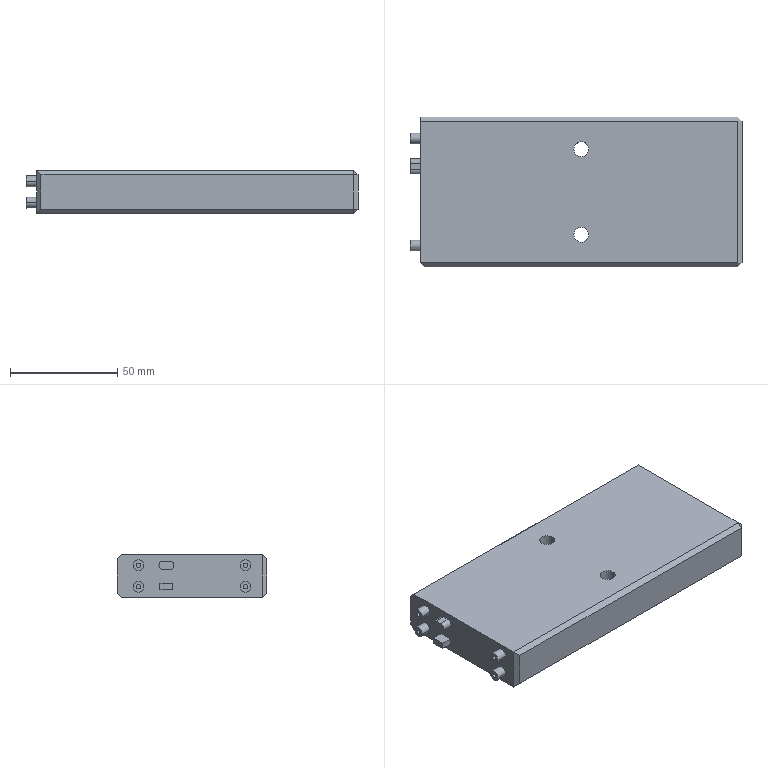Part | SolidWorks | features ICE 2, Chamfer 1, Extrusion 1 | 1 solid | 58 faces | box 155 x 70 x 20 mm | volume 207430 mm3 | plane 35 | cylinder 23 | commonest cylinder face diameters 2 x8 5 x8 7 x4 4 x3
STEP:
#1=CARTESIAN_POINT('',(-3.5,20.,-10.));
#2=VERTEX_POINT('',#1);
#3=CARTESIAN_POINT('',(3.5,20.,-10.));
#4=VERTEX_POINT('',#3);
#5=CARTESIAN_POINT('',(0.,20.,-10.));
#6=DIRECTION('',(0.,0.,1.));
#7=DIRECTION('',(1.,0.,0.));
#8=AXIS2_PLACEMENT_3D('',#5,#6,#7);
#9=CIRCLE('',#8,3.5);
#10=EDGE_CURVE('',#2,#4,#9,.T.);
#11=ORIENTED_EDGE('',*,*,#10,.F.);
#12=CARTESIAN_POINT('',(-3.5,20.,10.));
#13=VERTEX_POINT('',#12);
#14=CARTESIAN_POINT('',(-3.5,20.,-10.));
#15=DIRECTION('',(0.,0.,1.));
#16=VECTOR('',#15,1000.);
#17=LINE('',#14,#16);
#18=EDGE_CURVE('',#2,#13,#17,.T.);
#19=ORIENTED_EDGE('',*,*,#18,.T.);
#20=CARTESIAN_POINT('',(3.5,20.,10.));
#21=VERTEX_POINT('',#20);
#22=CARTESIAN_POINT('',(0.,20.,10.));
#23=DIRECTION('',(0.,0.,1.));
#24=DIRECTION('',(1.,0.,0.));
#25=AXIS2_PLACEMENT_3D('',#22,#23,#24);
#26=CIRCLE('',#25,3.5);
#27=EDGE_CURVE('',#13,#21,#26,.T.);
#28=ORIENTED_EDGE('',*,*,#27,.T.);
#29=CARTESIAN_POINT('',(3.5,20.,-10.));
#30=DIRECTION('',(0.,0.,1.));
#31=VECTOR('',#30,1000.);
#32=LINE('',#29,#31);
#33=EDGE_CURVE('',#4,#21,#32,.T.);
#34=ORIENTED_EDGE('',*,*,#33,.F.);
#35=EDGE_LOOP('',(#11,#19,#28,#34));
#36=FACE_OUTER_BOUND('',#35,.T.);
#37=CARTESIAN_POINT('',(0.,20.,-10.));
#38=DIRECTION('',(0.,0.,1.));
#39=DIRECTION('',(1.,0.,0.));
#40=AXIS2_PLACEMENT_3D('',#37,#38,#39);
#41=CYLINDRICAL_SURFACE('',#40,3.5);
#42=ADVANCED_FACE('',(#36),#41,.F.);
#43=CARTESIAN_POINT('',(-3.5,-20.,-10.));
#44=VERTEX_POINT('',#43);
#45=CARTESIAN_POINT('',(3.5,-20.,-10.));
#46=VERTEX_POINT('',#45);
#47=CARTESIAN_POINT('',(0.,-20.,-10.));
#48=DIRECTION('',(0.,0.,1.));
#49=DIRECTION('',(1.,0.,0.));
#50=AXIS2_PLACEMENT_3D('',#47,#48,#49);
#51=CIRCLE('',#50,3.5);
#52=EDGE_CURVE('',#44,#46,#51,.T.);
#53=ORIENTED_EDGE('',*,*,#52,.F.);
#54=CARTESIAN_POINT('',(-3.5,-20.,10.));
#55=VERTEX_POINT('',#54);
#56=CARTESIAN_POINT('',(-3.5,-20.,-10.));
#57=DIRECTION('',(0.,0.,1.));
#58=VECTOR('',#57,1000.);
#59=LINE('',#56,#58);
#60=EDGE_CURVE('',#44,#55,#59,.T.);
#61=ORIENTED_EDGE('',*,*,#60,.T.);
#62=CARTESIAN_POINT('',(3.5,-20.,10.));
#63=VERTEX_POINT('',#62);
#64=CARTESIAN_POINT('',(0.,-20.,10.));
#65=DIRECTION('',(0.,0.,1.));
#66=DIRECTION('',(1.,0.,0.));
#67=AXIS2_PLACEMENT_3D('',#64,#65,#66);
#68=CIRCLE('',#67,3.5);
#69=EDGE_CURVE('',#55,#63,#68,.T.);
#70=ORIENTED_EDGE('',*,*,#69,.T.);
#71=CARTESIAN_POINT('',(3.5,-20.,-10.));
#72=DIRECTION('',(0.,0.,1.));
#73=VECTOR('',#72,1000.);
#74=LINE('',#71,#73);
#75=EDGE_CURVE('',#46,#63,#74,.T.);
#76=ORIENTED_EDGE('',*,*,#75,.F.);
#77=EDGE_LOOP('',(#53,#61,#70,#76));
#78=FACE_OUTER_BOUND('',#77,.T.);
#79=CARTESIAN_POINT('',(0.,-20.,-10.));
#80=DIRECTION('',(0.,0.,1.));
#81=DIRECTION('',(1.,0.,0.));
#82=AXIS2_PLACEMENT_3D('',#79,#80,#81);
#83=CYLINDRICAL_SURFACE('',#82,3.5);
#84=ADVANCED_FACE('',(#78),#83,.F.);
#85=CARTESIAN_POINT('',(-80.,15.414,5.));
#86=VERTEX_POINT('',#85);
#87=CARTESIAN_POINT('',(-80.,13.414,3.));
#88=VERTEX_POINT('',#87);
#89=CARTESIAN_POINT('',(-80.,13.414,5.));
#90=DIRECTION('',(-1.,0.,0.));
#91=DIRECTION('',(0.,-1.,0.));
#92=AXIS2_PLACEMENT_3D('',#89,#90,#91);
#93=CIRCLE('',#92,2.);
#94=EDGE_CURVE('',#86,#88,#93,.T.);
#95=ORIENTED_EDGE('',*,*,#94,.F.);
#96=CARTESIAN_POINT('',(-75.,15.414,5.));
#97=VERTEX_POINT('',#96);
#98=CARTESIAN_POINT('',(-80.,15.414,5.));
#99=DIRECTION('',(1.,0.,0.));
#100=VECTOR('',#99,1000.);
#101=LINE('',#98,#100);
#102=EDGE_CURVE('',#86,#97,#101,.T.);
#103=ORIENTED_EDGE('',*,*,#102,.T.);
#104=CARTESIAN_POINT('',(-75.,13.414,3.));
#105=VERTEX_POINT('',#104);
#106=CARTESIAN_POINT('',(-75.,13.414,5.));
#107=DIRECTION('',(-1.,0.,0.));
#108=DIRECTION('',(0.,-1.,0.));
#109=AXIS2_PLACEMENT_3D('',#106,#107,#108);
#110=CIRCLE('',#109,2.);
#111=EDGE_CURVE('',#97,#105,#110,.T.);
#112=ORIENTED_EDGE('',*,*,#111,.T.);
#113=CARTESIAN_POINT('',(-80.,13.414,3.));
#114=DIRECTION('',(1.,0.,0.));
#115=VECTOR('',#114,1000.);
#116=LINE('',#113,#115);
#117=EDGE_CURVE('',#88,#105,#116,.T.);
#118=ORIENTED_EDGE('',*,*,#117,.F.);
#119=EDGE_LOOP('',(#95,#103,#112,#118));
#120=FACE_OUTER_BOUND('',#119,.T.);
#121=CARTESIAN_POINT('',(-80.,13.414,5.));
#122=DIRECTION('',(1.,0.,0.));
#123=DIRECTION('',(0.,1.,0.));
#124=AXIS2_PLACEMENT_3D('',#121,#122,#123);
#125=CYLINDRICAL_SURFACE('',#124,2.);
#126=ADVANCED_FACE('',(#120),#125,.T.);
#127=CARTESIAN_POINT('',(-80.,26.,-5.));
#128=VERTEX_POINT('',#127);
#129=CARTESIAN_POINT('',(-80.,24.,-5.));
#130=VERTEX_POINT('',#129);
#131=CARTESIAN_POINT('',(-80.,25.,-5.));
#132=DIRECTION('',(-1.,0.,0.));
#133=DIRECTION('',(0.,1.,0.));
#134=AXIS2_PLACEMENT_3D('',#131,#132,#133);
#135=CIRCLE('',#134,1.);
#136=EDGE_CURVE('',#128,#130,#135,.T.);
#137=ORIENTED_EDGE('',*,*,#136,.T.);
#138=CARTESIAN_POINT('',(-75.,24.,-5.));
#139=VERTEX_POINT('',#138);
#140=CARTESIAN_POINT('',(-80.,24.,-5.));
#141=DIRECTION('',(1.,0.,0.));
#142=VECTOR('',#141,1000.);
#143=LINE('',#140,#142);
#144=EDGE_CURVE('',#130,#139,#143,.T.);
#145=ORIENTED_EDGE('',*,*,#144,.T.);
#146=CARTESIAN_POINT('',(-75.,26.,-5.));
#147=VERTEX_POINT('',#146);
#148=CARTESIAN_POINT('',(-75.,25.,-5.));
#149=DIRECTION('',(-1.,0.,0.));
#150=DIRECTION('',(0.,1.,0.));
#151=AXIS2_PLACEMENT_3D('',#148,#149,#150);
#152=CIRCLE('',#151,1.);
#153=EDGE_CURVE('',#147,#139,#152,.T.);
#154=ORIENTED_EDGE('',*,*,#153,.F.);
#155=CARTESIAN_POINT('',(-80.,26.,-5.));
#156=DIRECTION('',(1.,0.,0.));
#157=VECTOR('',#156,1000.);
#158=LINE('',#155,#157);
#159=EDGE_CURVE('',#128,#147,#158,.T.);
#160=ORIENTED_EDGE('',*,*,#159,.F.);
#161=EDGE_LOOP('',(#137,#145,#154,#160));
#162=FACE_OUTER_BOUND('',#161,.T.);
#163=CARTESIAN_POINT('',(-80.,25.,-5.));
#164=DIRECTION('',(1.,0.,0.));
#165=DIRECTION('',(0.,1.,0.));
#166=AXIS2_PLACEMENT_3D('',#163,#164,#165);
#167=CYLINDRICAL_SURFACE('',#166,1.);
#168=ADVANCED_FACE('',(#162),#167,.F.);
#169=CARTESIAN_POINT('',(-80.,22.5,-5.));
#170=VERTEX_POINT('',#169);
#171=CARTESIAN_POINT('',(-80.,27.5,-5.));
#172=VERTEX_POINT('',#171);
#173=CARTESIAN_POINT('',(-80.,25.,-5.));
#174=DIRECTION('',(-1.,0.,0.));
#175=DIRECTION('',(0.,1.,0.));
#176=AXIS2_PLACEMENT_3D('',#173,#174,#175);
#177=CIRCLE('',#176,2.5);
#178=EDGE_CURVE('',#170,#172,#177,.T.);
#179=ORIENTED_EDGE('',*,*,#178,.F.);
#180=CARTESIAN_POINT('',(-75.,22.5,-5.));
#181=VERTEX_POINT('',#180);
#182=CARTESIAN_POINT('',(-80.,22.5,-5.));
#183=DIRECTION('',(1.,0.,0.));
#184=VECTOR('',#183,1000.);
#185=LINE('',#182,#184);
#186=EDGE_CURVE('',#170,#181,#185,.T.);
#187=ORIENTED_EDGE('',*,*,#186,.T.);
#188=CARTESIAN_POINT('',(-75.,27.5,-5.));
#189=VERTEX_POINT('',#188);
#190=CARTESIAN_POINT('',(-75.,25.,-5.));
#191=DIRECTION('',(-1.,0.,0.));
#192=DIRECTION('',(0.,1.,0.));
#193=AXIS2_PLACEMENT_3D('',#190,#191,#192);
#194=CIRCLE('',#193,2.5);
#195=EDGE_CURVE('',#181,#189,#194,.T.);
#196=ORIENTED_EDGE('',*,*,#195,.T.);
#197=CARTESIAN_POINT('',(-80.,27.5,-5.));
#198=DIRECTION('',(1.,0.,0.));
#199=VECTOR('',#198,1000.);
#200=LINE('',#197,#199);
#201=EDGE_CURVE('',#172,#189,#200,.T.);
#202=ORIENTED_EDGE('',*,*,#201,.F.);
#203=EDGE_LOOP('',(#179,#187,#196,#202));
#204=FACE_OUTER_BOUND('',#203,.T.);
#205=CARTESIAN_POINT('',(-80.,25.,-5.));
#206=DIRECTION('',(1.,0.,0.));
#207=DIRECTION('',(0.,1.,0.));
#208=AXIS2_PLACEMENT_3D('',#205,#206,#207);
#209=CYLINDRICAL_SURFACE('',#208,2.5);
#210=ADVANCED_FACE('',(#204),#209,.T.);
#211=CARTESIAN_POINT('',(-80.,26.,5.));
#212=VERTEX_POINT('',#211);
#213=CARTESIAN_POINT('',(-80.,24.,5.));
#214=VERTEX_POINT('',#213);
#215=CARTESIAN_POINT('',(-80.,25.,5.));
#216=DIRECTION('',(-1.,0.,0.));
#217=DIRECTION('',(0.,1.,0.));
#218=AXIS2_PLACEMENT_3D('',#215,#216,#217);
#219=CIRCLE('',#218,1.);
#220=EDGE_CURVE('',#212,#214,#219,.T.);
#221=ORIENTED_EDGE('',*,*,#220,.T.);
#222=CARTESIAN_POINT('',(-75.,24.,5.));
#223=VERTEX_POINT('',#222);
#224=CARTESIAN_POINT('',(-80.,24.,5.));
#225=DIRECTION('',(1.,0.,0.));
#226=VECTOR('',#225,1000.);
#227=LINE('',#224,#226);
#228=EDGE_CURVE('',#214,#223,#227,.T.);
#229=ORIENTED_EDGE('',*,*,#228,.T.);
#230=CARTESIAN_POINT('',(-75.,26.,5.));
#231=VERTEX_POINT('',#230);
#232=CARTESIAN_POINT('',(-75.,25.,5.));
#233=DIRECTION('',(-1.,0.,0.));
#234=DIRECTION('',(0.,1.,0.));
#235=AXIS2_PLACEMENT_3D('',#232,#233,#234);
#236=CIRCLE('',#235,1.);
#237=EDGE_CURVE('',#231,#223,#236,.T.);
#238=ORIENTED_EDGE('',*,*,#237,.F.);
#239=CARTESIAN_POINT('',(-80.,26.,5.));
#240=DIRECTION('',(1.,0.,0.));
#241=VECTOR('',#240,1000.);
#242=LINE('',#239,#241);
#243=EDGE_CURVE('',#212,#231,#242,.T.);
#244=ORIENTED_EDGE('',*,*,#243,.F.);
#245=EDGE_LOOP('',(#221,#229,#238,#244));
#246=FACE_OUTER_BOUND('',#245,.T.);
#247=CARTESIAN_POINT('',(-80.,25.,5.));
#248=DIRECTION('',(1.,0.,0.));
#249=DIRECTION('',(0.,1.,0.));
#250=AXIS2_PLACEMENT_3D('',#247,#248,#249);
#251=CYLINDRICAL_SURFACE('',#250,1.);
#252=ADVANCED_FACE('',(#246),#251,.F.);
#253=CARTESIAN_POINT('',(-80.,22.5,5.));
#254=VERTEX_POINT('',#253);
#255=CARTESIAN_POINT('',(-80.,27.5,5.));
#256=VERTEX_POINT('',#255);
#257=CARTESIAN_POINT('',(-80.,25.,5.));
#258=DIRECTION('',(-1.,0.,0.));
#259=DIRECTION('',(0.,1.,0.));
#260=AXIS2_PLACEMENT_3D('',#257,#258,#259);
#261=CIRCLE('',#260,2.5);
#262=EDGE_CURVE('',#254,#256,#261,.T.);
#263=ORIENTED_EDGE('',*,*,#262,.F.);
#264=CARTESIAN_POINT('',(-75.,22.5,5.));
#265=VERTEX_POINT('',#264);
#266=CARTESIAN_POINT('',(-80.,22.5,5.));
#267=DIRECTION('',(1.,0.,0.));
#268=VECTOR('',#267,1000.);
#269=LINE('',#266,#268);
#270=EDGE_CURVE('',#254,#265,#269,.T.);
#271=ORIENTED_EDGE('',*,*,#270,.T.);
#272=CARTESIAN_POINT('',(-75.,27.5,5.));
#273=VERTEX_POINT('',#272);
#274=CARTESIAN_POINT('',(-75.,25.,5.));
#275=DIRECTION('',(-1.,0.,0.));
#276=DIRECTION('',(0.,1.,0.));
#277=AXIS2_PLACEMENT_3D('',#274,#275,#276);
#278=CIRCLE('',#277,2.5);
#279=EDGE_CURVE('',#265,#273,#278,.T.);
#280=ORIENTED_EDGE('',*,*,#279,.T.);
#281=CARTESIAN_POINT('',(-80.,27.5,5.));
#282=DIRECTION('',(1.,0.,0.));
#283=VECTOR('',#282,1000.);
#284=LINE('',#281,#283);
#285=EDGE_CURVE('',#256,#273,#284,.T.);
#286=ORIENTED_EDGE('',*,*,#285,.F.);
#287=EDGE_LOOP('',(#263,#271,#280,#286));
#288=FACE_OUTER_BOUND('',#287,.T.);
#289=CARTESIAN_POINT('',(-80.,25.,5.));
#290=DIRECTION('',(1.,0.,0.));
#291=DIRECTION('',(0.,1.,0.));
#292=AXIS2_PLACEMENT_3D('',#289,#290,#291);
#293=CYLINDRICAL_SURFACE('',#292,2.5);
#294=ADVANCED_FACE('',(#288),#293,.T.);
#295=CARTESIAN_POINT('',(-80.,-24.,5.));
#296=VERTEX_POINT('',#295);
#297=CARTESIAN_POINT('',(-80.,-26.,5.));
#298=VERTEX_POINT('',#297);
#299=CARTESIAN_POINT('',(-80.,-25.,5.));
#300=DIRECTION('',(-1.,0.,0.));
#301=DIRECTION('',(0.,-1.,0.));
#302=AXIS2_PLACEMENT_3D('',#299,#300,#301);
#303=CIRCLE('',#302,1.);
#304=EDGE_CURVE('',#296,#298,#303,.T.);
#305=ORIENTED_EDGE('',*,*,#304,.T.);
#306=CARTESIAN_POINT('',(-75.,-26.,5.));
#307=VERTEX_POINT('',#306);
#308=CARTESIAN_POINT('',(-80.,-26.,5.));
#309=DIRECTION('',(1.,0.,0.));
#310=VECTOR('',#309,1000.);
#311=LINE('',#308,#310);
#312=EDGE_CURVE('',#298,#307,#311,.T.);
#313=ORIENTED_EDGE('',*,*,#312,.T.);
#314=CARTESIAN_POINT('',(-75.,-24.,5.));
#315=VERTEX_POINT('',#314);
#316=CARTESIAN_POINT('',(-75.,-25.,5.));
#317=DIRECTION('',(-1.,0.,0.));
#318=DIRECTION('',(0.,-1.,0.));
#319=AXIS2_PLACEMENT_3D('',#316,#317,#318);
#320=CIRCLE('',#319,1.);
#321=EDGE_CURVE('',#315,#307,#320,.T.);
#322=ORIENTED_EDGE('',*,*,#321,.F.);
#323=CARTESIAN_POINT('',(-80.,-24.,5.));
#324=DIRECTION('',(1.,0.,0.));
#325=VECTOR('',#324,1000.);
#326=LINE('',#323,#325);
#327=EDGE_CURVE('',#296,#315,#326,.T.);
#328=ORIENTED_EDGE('',*,*,#327,.F.);
#329=EDGE_LOOP('',(#305,#313,#322,#328));
#330=FACE_OUTER_BOUND('',#329,.T.);
#331=CARTESIAN_POINT('',(-80.,-25.,5.));
#332=DIRECTION('',(1.,0.,0.));
#333=DIRECTION('',(0.,1.,0.));
#334=AXIS2_PLACEMENT_3D('',#331,#332,#333);
#335=CYLINDRICAL_SURFACE('',#334,1.);
#336=ADVANCED_FACE('',(#330),#335,.F.);
#337=CARTESIAN_POINT('',(-80.,-27.5,5.));
#338=VERTEX_POINT('',#337);
#339=CARTESIAN_POINT('',(-80.,-22.5,5.));
#340=VERTEX_POINT('',#339);
#341=CARTESIAN_POINT('',(-80.,-25.,5.));
#342=DIRECTION('',(-1.,0.,0.));
#343=DIRECTION('',(0.,-1.,0.));
#344=AXIS2_PLACEMENT_3D('',#341,#342,#343);
#345=CIRCLE('',#344,2.5);
#346=EDGE_CURVE('',#338,#340,#345,.T.);
#347=ORIENTED_EDGE('',*,*,#346,.F.);
#348=CARTESIAN_POINT('',(-75.,-27.5,5.));
#349=VERTEX_POINT('',#348);
#350=CARTESIAN_POINT('',(-80.,-27.5,5.));
#351=DIRECTION('',(1.,0.,0.));
#352=VECTOR('',#351,1000.);
#353=LINE('',#350,#352);
#354=EDGE_CURVE('',#338,#349,#353,.T.);
#355=ORIENTED_EDGE('',*,*,#354,.T.);
#356=CARTESIAN_POINT('',(-75.,-22.5,5.));
#357=VERTEX_POINT('',#356);
#358=CARTESIAN_POINT('',(-75.,-25.,5.));
#359=DIRECTION('',(-1.,0.,0.));
#360=DIRECTION('',(0.,1.,0.));
#361=AXIS2_PLACEMENT_3D('',#358,#359,#360);
#362=CIRCLE('',#361,2.5);
#363=EDGE_CURVE('',#349,#357,#362,.T.);
#364=ORIENTED_EDGE('',*,*,#363,.T.);
#365=CARTESIAN_POINT('',(-80.,-22.5,5.));
#366=DIRECTION('',(1.,0.,0.));
#367=VECTOR('',#366,1000.);
#368=LINE('',#365,#367);
#369=EDGE_CURVE('',#340,#357,#368,.T.);
#370=ORIENTED_EDGE('',*,*,#369,.F.);
#371=EDGE_LOOP('',(#347,#355,#364,#370));
#372=FACE_OUTER_BOUND('',#371,.T.);
#373=CARTESIAN_POINT('',(-80.,-25.,5.));
#374=DIRECTION('',(1.,0.,0.));
#375=DIRECTION('',(0.,1.,0.));
#376=AXIS2_PLACEMENT_3D('',#373,#374,#375);
#377=CYLINDRICAL_SURFACE('',#376,2.5);
#378=ADVANCED_FACE('',(#372),#377,.T.);
#379=CARTESIAN_POINT('',(-80.,-24.,-5.));
#380=VERTEX_POINT('',#379);
#381=CARTESIAN_POINT('',(-80.,-26.,-5.));
#382=VERTEX_POINT('',#381);
#383=CARTESIAN_POINT('',(-80.,-25.,-5.));
#384=DIRECTION('',(-1.,0.,0.));
#385=DIRECTION('',(0.,-1.,0.));
#386=AXIS2_PLACEMENT_3D('',#383,#384,#385);
#387=CIRCLE('',#386,1.);
#388=EDGE_CURVE('',#380,#382,#387,.T.);
#389=ORIENTED_EDGE('',*,*,#388,.T.);
#390=CARTESIAN_POINT('',(-75.,-26.,-5.));
#391=VERTEX_POINT('',#390);
#392=CARTESIAN_POINT('',(-80.,-26.,-5.));
#393=DIRECTION('',(1.,0.,0.));
#394=VECTOR('',#393,1000.);
#395=LINE('',#392,#394);
#396=EDGE_CURVE('',#382,#391,#395,.T.);
#397=ORIENTED_EDGE('',*,*,#396,.T.);
#398=CARTESIAN_POINT('',(-75.,-24.,-5.));
#399=VERTEX_POINT('',#398);
#400=CARTESIAN_POINT('',(-75.,-25.,-5.));
#401=DIRECTION('',(-1.,0.,0.));
#402=DIRECTION('',(0.,-1.,0.));
#403=AXIS2_PLACEMENT_3D('',#400,#401,#402);
#404=CIRCLE('',#403,1.);
#405=EDGE_CURVE('',#399,#391,#404,.T.);
#406=ORIENTED_EDGE('',*,*,#405,.F.);
#407=CARTESIAN_POINT('',(-80.,-24.,-5.));
#408=DIRECTION('',(1.,0.,0.));
#409=VECTOR('',#408,1000.);
#410=LINE('',#407,#409);
#411=EDGE_CURVE('',#380,#399,#410,.T.);
#412=ORIENTED_EDGE('',*,*,#411,.F.);
#413=EDGE_LOOP('',(#389,#397,#406,#412));
#414=FACE_OUTER_BOUND('',#413,.T.);
#415=CARTESIAN_POINT('',(-80.,-25.,-5.));
#416=DIRECTION('',(1.,0.,0.));
#417=DIRECTION('',(0.,1.,0.));
#418=AXIS2_PLACEMENT_3D('',#415,#416,#417);
#419=CYLINDRICAL_SURFACE('',#418,1.);
#420=ADVANCED_FACE('',(#414),#419,.F.);
#421=CARTESIAN_POINT('',(-80.,-27.5,-5.));
#422=VERTEX_POINT('',#421);
#423=CARTESIAN_POINT('',(-80.,-22.5,-5.));
#424=VERTEX_POINT('',#423);
#425=CARTESIAN_POINT('',(-80.,-25.,-5.));
#426=DIRECTION('',(-1.,0.,0.));
#427=DIRECTION('',(0.,-1.,0.));
#428=AXIS2_PLACEMENT_3D('',#425,#426,#427);
#429=CIRCLE('',#428,2.5);
#430=EDGE_CURVE('',#422,#424,#429,.T.);
#431=ORIENTED_EDGE('',*,*,#430,.F.);
#432=CARTESIAN_POINT('',(-75.,-27.5,-5.));
#433=VERTEX_POINT('',#432);
#434=CARTESIAN_POINT('',(-80.,-27.5,-5.));
#435=DIRECTION('',(1.,0.,0.));
#436=VECTOR('',#435,1000.);
#437=LINE('',#434,#436);
#438=EDGE_CURVE('',#422,#433,#437,.T.);
#439=ORIENTED_EDGE('',*,*,#438,.T.);
#440=CARTESIAN_POINT('',(-75.,-22.5,-5.));
#441=VERTEX_POINT('',#440);
#442=CARTESIAN_POINT('',(-75.,-25.,-5.));
#443=DIRECTION('',(-1.,0.,0.));
#444=DIRECTION('',(0.,1.,0.));
#445=AXIS2_PLACEMENT_3D('',#442,#443,#444);
#446=CIRCLE('',#445,2.5);
#447=EDGE_CURVE('',#433,#441,#446,.T.);
#448=ORIENTED_EDGE('',*,*,#447,.T.);
#449=CARTESIAN_POINT('',(-80.,-22.5,-5.));
#450=DIRECTION('',(1.,0.,0.));
#451=VECTOR('',#450,1000.);
#452=LINE('',#449,#451);
#453=EDGE_CURVE('',#424,#441,#452,.T.);
#454=ORIENTED_EDGE('',*,*,#453,.F.);
#455=EDGE_LOOP('',(#431,#439,#448,#454));
#456=FACE_OUTER_BOUND('',#455,.T.);
#457=CARTESIAN_POINT('',(-80.,-25.,-5.));
#458=DIRECTION('',(1.,0.,0.));
#459=DIRECTION('',(0.,1.,0.));
#460=AXIS2_PLACEMENT_3D('',#457,#458,#459);
#461=CYLINDRICAL_SURFACE('',#460,2.5);
#462=ADVANCED_FACE('',(#456),#461,.T.);
#463=CARTESIAN_POINT('',(-75.,13.414,7.));
#464=VERTEX_POINT('',#463);
#465=CARTESIAN_POINT('',(-75.,13.414,5.));
#466=DIRECTION('',(-1.,0.,0.));
#467=DIRECTION('',(0.,-1.,0.));
#468=AXIS2_PLACEMENT_3D('',#465,#466,#467);
#469=CIRCLE('',#468,2.);
#470=EDGE_CURVE('',#464,#97,#469,.T.);
#471=ORIENTED_EDGE('',*,*,#470,.F.);
#472=CARTESIAN_POINT('',(-75.,10.414,7.));
#473=VERTEX_POINT('',#472);
#474=CARTESIAN_POINT('',(-75.,13.414,7.));
#475=DIRECTION('',(0.,1.,0.));
#476=VECTOR('',#475,1000.);
#477=LINE('',#474,#476);
#478=EDGE_CURVE('',#473,#464,#477,.T.);
#479=ORIENTED_EDGE('',*,*,#478,.F.);
#480=CARTESIAN_POINT('',(-75.,10.414,3.));
#481=VERTEX_POINT('',#480);
#482=CARTESIAN_POINT('',(-75.,10.414,5.));
#483=DIRECTION('',(-1.,0.,0.));
#484=DIRECTION('',(0.,-1.,0.));
#485=AXIS2_PLACEMENT_3D('',#482,#483,#484);
#486=CIRCLE('',#485,2.);
#487=EDGE_CURVE('',#481,#473,#486,.T.);
#488=ORIENTED_EDGE('',*,*,#487,.F.);
#489=CARTESIAN_POINT('',(-75.,13.414,3.));
#490=DIRECTION('',(0.,-1.,0.));
#491=VECTOR('',#490,1000.);
#492=LINE('',#489,#491);
#493=EDGE_CURVE('',#105,#481,#492,.T.);
#494=ORIENTED_EDGE('',*,*,#493,.F.);
#495=ORIENTED_EDGE('',*,*,#111,.F.);
#496=EDGE_LOOP('',(#471,#479,#488,#494,#495));
#497=FACE_BOUND('',#496,.T.);
#498=CARTESIAN_POINT('',(-75.,25.,-5.));
#499=DIRECTION('',(-1.,0.,0.));
#500=DIRECTION('',(0.,1.,0.));
#501=AXIS2_PLACEMENT_3D('',#498,#499,#500);
#502=CIRCLE('',#501,2.5);
#503=EDGE_CURVE('',#189,#181,#502,.T.);
#504=ORIENTED_EDGE('',*,*,#503,.F.);
#505=ORIENTED_EDGE('',*,*,#195,.F.);
#506=EDGE_LOOP('',(#504,#505));
#507=FACE_BOUND('',#506,.T.);
#508=CARTESIAN_POINT('',(-75.,25.,5.));
#509=DIRECTION('',(-1.,0.,0.));
#510=DIRECTION('',(0.,1.,0.));
#511=AXIS2_PLACEMENT_3D('',#508,#509,#510);
#512=CIRCLE('',#511,2.5);
#513=EDGE_CURVE('',#273,#265,#512,.T.);
#514=ORIENTED_EDGE('',*,*,#513,.F.);
#515=ORIENTED_EDGE('',*,*,#279,.F.);
#516=EDGE_LOOP('',(#514,#515));
#517=FACE_BOUND('',#516,.T.);
#518=CARTESIAN_POINT('',(-75.,-25.,5.));
#519=DIRECTION('',(-1.,0.,0.));
#520=DIRECTION('',(0.,1.,0.));
#521=AXIS2_PLACEMENT_3D('',#518,#519,#520);
#522=CIRCLE('',#521,2.5);
#523=EDGE_CURVE('',#357,#349,#522,.T.);
#524=ORIENTED_EDGE('',*,*,#523,.F.);
#525=ORIENTED_EDGE('',*,*,#363,.F.);
#526=EDGE_LOOP('',(#524,#525));
#527=FACE_BOUND('',#526,.T.);
#528=CARTESIAN_POINT('',(-75.,-25.,-5.));
#529=DIRECTION('',(-1.,0.,0.));
#530=DIRECTION('',(0.,1.,0.));
#531=AXIS2_PLACEMENT_3D('',#528,#529,#530);
#532=CIRCLE('',#531,2.5);
#533=EDGE_CURVE('',#441,#433,#532,.T.);
#534=ORIENTED_EDGE('',*,*,#533,.F.);
#535=ORIENTED_EDGE('',*,*,#447,.F.);
#536=EDGE_LOOP('',(#534,#535));
#537=FACE_BOUND('',#536,.T.);
#538=CARTESIAN_POINT('',(-75.,35.,8.));
#539=VERTEX_POINT('',#538);
#540=CARTESIAN_POINT('',(-75.,35.,-8.));
#541=VERTEX_POINT('',#540);
#542=CARTESIAN_POINT('',(-75.,35.,10.));
#543=DIRECTION('',(0.,0.,-1.));
#544=VECTOR('',#543,1000.);
#545=LINE('',#542,#544);
#546=EDGE_CURVE('',#539,#541,#545,.T.);
#547=ORIENTED_EDGE('',*,*,#546,.T.);
#548=CARTESIAN_POINT('',(-75.,33.,-10.));
#549=VERTEX_POINT('',#548);
#550=CARTESIAN_POINT('',(-75.,35.,-8.));
#551=DIRECTION('',(0.,-0.7071,-0.7071));
#552=VECTOR('',#551,1000.);
#553=LINE('',#550,#552);
#554=EDGE_CURVE('',#541,#549,#553,.T.);
#555=ORIENTED_EDGE('',*,*,#554,.T.);
#556=CARTESIAN_POINT('',(-75.,-33.,-10.));
#557=VERTEX_POINT('',#556);
#558=CARTESIAN_POINT('',(-75.,35.,-10.));
#559=DIRECTION('',(0.,-1.,0.));
#560=VECTOR('',#559,1000.);
#561=LINE('',#558,#560);
#562=EDGE_CURVE('',#549,#557,#561,.T.);
#563=ORIENTED_EDGE('',*,*,#562,.T.);
#564=CARTESIAN_POINT('',(-75.,-33.,10.));
#565=VERTEX_POINT('',#564);
#566=CARTESIAN_POINT('',(-75.,-33.,10.));
#567=DIRECTION('',(0.,0.,1.));
#568=VECTOR('',#567,1000.);
#569=LINE('',#566,#568);
#570=EDGE_CURVE('',#557,#565,#569,.T.);
#571=ORIENTED_EDGE('',*,*,#570,.T.);
#572=CARTESIAN_POINT('',(-75.,33.,10.));
#573=VERTEX_POINT('',#572);
#574=CARTESIAN_POINT('',(-75.,35.,10.));
#575=DIRECTION('',(0.,-1.,0.));
#576=VECTOR('',#575,1000.);
#577=LINE('',#574,#576);
#578=EDGE_CURVE('',#573,#565,#577,.T.);
#579=ORIENTED_EDGE('',*,*,#578,.F.);
#580=CARTESIAN_POINT('',(-75.,33.,10.));
#581=DIRECTION('',(0.,0.7071,-0.7071));
#582=VECTOR('',#581,1000.);
#583=LINE('',#580,#582);
#584=EDGE_CURVE('',#573,#539,#583,.T.);
#585=ORIENTED_EDGE('',*,*,#584,.T.);
#586=EDGE_LOOP('',(#547,#555,#563,#571,#579,#585));
#587=FACE_OUTER_BOUND('',#586,.T.);
#588=CARTESIAN_POINT('',(-75.,15.,-6.5));
#589=VERTEX_POINT('',#588);
#590=CARTESIAN_POINT('',(-75.,9.,-6.5));
#591=VERTEX_POINT('',#590);
#592=CARTESIAN_POINT('',(-75.,15.,-6.5));
#593=DIRECTION('',(0.,-1.,0.));
#594=VECTOR('',#593,1000.);
#595=LINE('',#592,#594);
#596=EDGE_CURVE('',#589,#591,#595,.T.);
#597=ORIENTED_EDGE('',*,*,#596,.F.);
#598=CARTESIAN_POINT('',(-75.,15.,-3.5));
#599=VERTEX_POINT('',#598);
#600=CARTESIAN_POINT('',(-75.,15.,-6.5));
#601=DIRECTION('',(0.,0.,-1.));
#602=VECTOR('',#601,1000.);
#603=LINE('',#600,#602);
#604=EDGE_CURVE('',#599,#589,#603,.T.);
#605=ORIENTED_EDGE('',*,*,#604,.F.);
#606=CARTESIAN_POINT('',(-75.,9.,-3.5));
#607=VERTEX_POINT('',#606);
#608=CARTESIAN_POINT('',(-75.,15.,-3.5));
#609=DIRECTION('',(0.,1.,0.));
#610=VECTOR('',#609,1000.);
#611=LINE('',#608,#610);
#612=EDGE_CURVE('',#607,#599,#611,.T.);
#613=ORIENTED_EDGE('',*,*,#612,.F.);
#614=CARTESIAN_POINT('',(-75.,9.,-6.5));
#615=DIRECTION('',(0.,0.,1.));
#616=VECTOR('',#615,1000.);
#617=LINE('',#614,#616);
#618=EDGE_CURVE('',#591,#607,#617,.T.);
#619=ORIENTED_EDGE('',*,*,#618,.F.);
#620=EDGE_LOOP('',(#597,#605,#613,#619));
#621=FACE_BOUND('',#620,.T.);
#622=CARTESIAN_POINT('',(-75.,35.,10.));
#623=DIRECTION('',(1.,0.,0.));
#624=DIRECTION('',(0.,1.,0.));
#625=AXIS2_PLACEMENT_3D('',#622,#623,#624);
#626=PLANE('',#625);
#627=ADVANCED_FACE('',(#497,#507,#517,#527,#537,#587,#621),#626,.F.);
#628=CARTESIAN_POINT('',(75.,33.,8.));
#629=VERTEX_POINT('',#628);
#630=CARTESIAN_POINT('',(75.,-33.,8.));
#631=VERTEX_POINT('',#630);
#632=CARTESIAN_POINT('',(75.,-35.,8.));
#633=DIRECTION('',(0.,-1.,0.));
#634=VECTOR('',#633,1000.);
#635=LINE('',#632,#634);
#636=EDGE_CURVE('',#629,#631,#635,.T.);
#637=ORIENTED_EDGE('',*,*,#636,.T.);
#638=CARTESIAN_POINT('',(75.,-33.,-8.));
#639=VERTEX_POINT('',#638);
#640=CARTESIAN_POINT('',(75.,-33.,10.));
#641=DIRECTION('',(0.,0.,-1.));
#642=VECTOR('',#641,1000.);
#643=LINE('',#640,#642);
#644=EDGE_CURVE('',#631,#639,#643,.T.);
#645=ORIENTED_EDGE('',*,*,#644,.T.);
#646=CARTESIAN_POINT('',(75.,33.,-8.));
#647=VERTEX_POINT('',#646);
#648=CARTESIAN_POINT('',(75.,35.,-8.));
#649=DIRECTION('',(0.,1.,0.));
#650=VECTOR('',#649,1000.);
#651=LINE('',#648,#650);
#652=EDGE_CURVE('',#639,#647,#651,.T.);
#653=ORIENTED_EDGE('',*,*,#652,.T.);
#654=CARTESIAN_POINT('',(75.,33.,10.));
#655=DIRECTION('',(0.,0.,1.));
#656=VECTOR('',#655,1000.);
#657=LINE('',#654,#656);
#658=EDGE_CURVE('',#647,#629,#657,.T.);
#659=ORIENTED_EDGE('',*,*,#658,.T.);
#660=EDGE_LOOP('',(#637,#645,#653,#659));
#661=FACE_OUTER_BOUND('',#660,.T.);
#662=CARTESIAN_POINT('',(75.,35.,10.));
#663=DIRECTION('',(-1.,0.,0.));
#664=DIRECTION('',(0.,-1.,0.));
#665=AXIS2_PLACEMENT_3D('',#662,#663,#664);
#666=PLANE('',#665);
#667=ADVANCED_FACE('',(#661),#666,.F.);
#668=CARTESIAN_POINT('',(73.,35.,8.));
#669=VERTEX_POINT('',#668);
#670=CARTESIAN_POINT('',(73.,35.,-8.));
#671=VERTEX_POINT('',#670);
#672=CARTESIAN_POINT('',(73.,35.,10.));
#673=DIRECTION('',(0.,0.,-1.));
#674=VECTOR('',#673,1000.);
#675=LINE('',#672,#674);
#676=EDGE_CURVE('',#669,#671,#675,.T.);
#677=ORIENTED_EDGE('',*,*,#676,.T.);
#678=CARTESIAN_POINT('',(-75.,35.,-8.));
#679=DIRECTION('',(-1.,0.,0.));
#680=VECTOR('',#679,1000.);
#681=LINE('',#678,#680);
#682=EDGE_CURVE('',#671,#541,#681,.T.);
#683=ORIENTED_EDGE('',*,*,#682,.T.);
#684=ORIENTED_EDGE('',*,*,#546,.F.);
#685=CARTESIAN_POINT('',(75.,35.,8.));
#686=DIRECTION('',(1.,0.,0.));
#687=VECTOR('',#686,1000.);
#688=LINE('',#685,#687);
#689=EDGE_CURVE('',#539,#669,#688,.T.);
#690=ORIENTED_EDGE('',*,*,#689,.T.);
#691=EDGE_LOOP('',(#677,#683,#684,#690));
#692=FACE_OUTER_BOUND('',#691,.T.);
#693=CARTESIAN_POINT('',(-75.,35.,10.));
#694=DIRECTION('',(0.,-1.,0.));
#695=DIRECTION('',(0.,0.,-1.));
#696=AXIS2_PLACEMENT_3D('',#693,#694,#695);
#697=PLANE('',#696);
#698=ADVANCED_FACE('',(#692),#697,.F.);
#699=CARTESIAN_POINT('',(-73.,-35.,-8.));
#700=VERTEX_POINT('',#699);
#701=CARTESIAN_POINT('',(73.,-35.,-8.));
#702=VERTEX_POINT('',#701);
#703=CARTESIAN_POINT('',(-75.,-35.,-8.));
#704=DIRECTION('',(1.,0.,0.));
#705=VECTOR('',#704,1000.);
#706=LINE('',#703,#705);
#707=EDGE_CURVE('',#700,#702,#706,.T.);
#708=ORIENTED_EDGE('',*,*,#707,.T.);
#709=CARTESIAN_POINT('',(73.,-35.,8.));
#710=VERTEX_POINT('',#709);
#711=CARTESIAN_POINT('',(73.,-35.,10.));
#712=DIRECTION('',(0.,0.,1.));
#713=VECTOR('',#712,1000.);
#714=LINE('',#711,#713);
#715=EDGE_CURVE('',#702,#710,#714,.T.);
#716=ORIENTED_EDGE('',*,*,#715,.T.);
#717=CARTESIAN_POINT('',(-73.,-35.,8.));
#718=VERTEX_POINT('',#717);
#719=CARTESIAN_POINT('',(-75.,-35.,8.));
#720=DIRECTION('',(-1.,0.,0.));
#721=VECTOR('',#720,1000.);
#722=LINE('',#719,#721);
#723=EDGE_CURVE('',#710,#718,#722,.T.);
#724=ORIENTED_EDGE('',*,*,#723,.T.);
#725=CARTESIAN_POINT('',(-73.,-35.,10.));
#726=DIRECTION('',(0.,0.,-1.));
#727=VECTOR('',#726,1000.);
#728=LINE('',#725,#727);
#729=EDGE_CURVE('',#718,#700,#728,.T.);
#730=ORIENTED_EDGE('',*,*,#729,.T.);
#731=EDGE_LOOP('',(#708,#716,#724,#730));
#732=FACE_OUTER_BOUND('',#731,.T.);
#733=CARTESIAN_POINT('',(-75.,-35.,10.));
#734=DIRECTION('',(0.,1.,0.));
#735=DIRECTION('',(0.,0.,1.));
#736=AXIS2_PLACEMENT_3D('',#733,#734,#735);
#737=PLANE('',#736);
#738=ADVANCED_FACE('',(#732),#737,.F.);
#739=CARTESIAN_POINT('',(0.,20.,10.));
#740=DIRECTION('',(0.,0.,1.));
#741=DIRECTION('',(1.,0.,0.));
#742=AXIS2_PLACEMENT_3D('',#739,#740,#741);
#743=CIRCLE('',#742,3.5);
#744=EDGE_CURVE('',#21,#13,#743,.T.);
#745=ORIENTED_EDGE('',*,*,#744,.F.);
#746=ORIENTED_EDGE('',*,*,#27,.F.);
#747=EDGE_LOOP('',(#745,#746));
#748=FACE_BOUND('',#747,.T.);
#749=CARTESIAN_POINT('',(0.,-20.,10.));
#750=DIRECTION('',(0.,0.,1.));
#751=DIRECTION('',(1.,0.,0.));
#752=AXIS2_PLACEMENT_3D('',#749,#750,#751);
#753=CIRCLE('',#752,3.5);
#754=EDGE_CURVE('',#63,#55,#753,.T.);
#755=ORIENTED_EDGE('',*,*,#754,.F.);
#756=ORIENTED_EDGE('',*,*,#69,.F.);
#757=EDGE_LOOP('',(#755,#756));
#758=FACE_BOUND('',#757,.T.);
#759=CARTESIAN_POINT('',(73.,-33.,10.));
#760=VERTEX_POINT('',#759);
#761=CARTESIAN_POINT('',(73.,33.,10.));
#762=VERTEX_POINT('',#761);
#763=CARTESIAN_POINT('',(73.,35.,10.));
#764=DIRECTION('',(0.,1.,0.));
#765=VECTOR('',#764,1000.);
#766=LINE('',#763,#765);
#767=EDGE_CURVE('',#760,#762,#766,.T.);
#768=ORIENTED_EDGE('',*,*,#767,.T.);
#769=CARTESIAN_POINT('',(-75.,33.,10.));
#770=DIRECTION('',(-1.,0.,0.));
#771=VECTOR('',#770,1000.);
#772=LINE('',#769,#771);
#773=EDGE_CURVE('',#762,#573,#772,.T.);
#774=ORIENTED_EDGE('',*,*,#773,.T.);
#775=ORIENTED_EDGE('',*,*,#578,.T.);
#776=CARTESIAN_POINT('',(75.,-33.,10.));
#777=DIRECTION('',(1.,0.,0.));
#778=VECTOR('',#777,1000.);
#779=LINE('',#776,#778);
#780=EDGE_CURVE('',#565,#760,#779,.T.);
#781=ORIENTED_EDGE('',*,*,#780,.T.);
#782=EDGE_LOOP('',(#768,#774,#775,#781));
#783=FACE_OUTER_BOUND('',#782,.T.);
#784=CARTESIAN_POINT('',(0.,0.,10.));
#785=DIRECTION('',(0.,0.,1.));
#786=DIRECTION('',(1.,0.,0.));
#787=AXIS2_PLACEMENT_3D('',#784,#785,#786);
#788=PLANE('',#787);
#789=ADVANCED_FACE('',(#748,#758,#783),#788,.T.);
#790=CARTESIAN_POINT('',(0.,20.,-10.));
#791=DIRECTION('',(0.,0.,1.));
#792=DIRECTION('',(1.,0.,0.));
#793=AXIS2_PLACEMENT_3D('',#790,#791,#792);
#794=CIRCLE('',#793,3.5);
#795=EDGE_CURVE('',#4,#2,#794,.T.);
#796=ORIENTED_EDGE('',*,*,#795,.T.);
#797=ORIENTED_EDGE('',*,*,#10,.T.);
#798=EDGE_LOOP('',(#796,#797));
#799=FACE_BOUND('',#798,.T.);
#800=CARTESIAN_POINT('',(0.,-20.,-10.));
#801=DIRECTION('',(0.,0.,1.));
#802=DIRECTION('',(1.,0.,0.));
#803=AXIS2_PLACEMENT_3D('',#800,#801,#802);
#804=CIRCLE('',#803,3.5);
#805=EDGE_CURVE('',#46,#44,#804,.T.);
#806=ORIENTED_EDGE('',*,*,#805,.T.);
#807=ORIENTED_EDGE('',*,*,#52,.T.);
#808=EDGE_LOOP('',(#806,#807));
#809=FACE_BOUND('',#808,.T.);
#810=ORIENTED_EDGE('',*,*,#562,.F.);
#811=CARTESIAN_POINT('',(73.,33.,-10.));
#812=VERTEX_POINT('',#811);
#813=CARTESIAN_POINT('',(0.,33.,-10.));
#814=DIRECTION('',(1.,0.,0.));
#815=VECTOR('',#814,1000.);
#816=LINE('',#813,#815);
#817=EDGE_CURVE('',#549,#812,#816,.T.);
#818=ORIENTED_EDGE('',*,*,#817,.T.);
#819=CARTESIAN_POINT('',(73.,-33.,-10.));
#820=VERTEX_POINT('',#819);
#821=CARTESIAN_POINT('',(73.,0.,-10.));
#822=DIRECTION('',(0.,-1.,0.));
#823=VECTOR('',#822,1000.);
#824=LINE('',#821,#823);
#825=EDGE_CURVE('',#812,#820,#824,.T.);
#826=ORIENTED_EDGE('',*,*,#825,.T.);
#827=CARTESIAN_POINT('',(0.,-33.,-10.));
#828=DIRECTION('',(-1.,0.,0.));
#829=VECTOR('',#828,1000.);
#830=LINE('',#827,#829);
#831=EDGE_CURVE('',#820,#557,#830,.T.);
#832=ORIENTED_EDGE('',*,*,#831,.T.);
#833=EDGE_LOOP('',(#810,#818,#826,#832));
#834=FACE_OUTER_BOUND('',#833,.T.);
#835=CARTESIAN_POINT('',(0.,0.,-10.));
#836=DIRECTION('',(0.,0.,1.));
#837=DIRECTION('',(1.,0.,0.));
#838=AXIS2_PLACEMENT_3D('',#835,#836,#837);
#839=PLANE('',#838);
#840=ADVANCED_FACE('',(#799,#809,#834),#839,.F.);
#841=CARTESIAN_POINT('',(-80.,-25.,-5.));
#842=DIRECTION('',(-1.,0.,0.));
#843=DIRECTION('',(0.,-1.,0.));
#844=AXIS2_PLACEMENT_3D('',#841,#842,#843);
#845=CIRCLE('',#844,2.5);
#846=EDGE_CURVE('',#424,#422,#845,.T.);
#847=ORIENTED_EDGE('',*,*,#846,.T.);
#848=ORIENTED_EDGE('',*,*,#430,.T.);
#849=EDGE_LOOP('',(#847,#848));
#850=FACE_OUTER_BOUND('',#849,.T.);
#851=ORIENTED_EDGE('',*,*,#388,.F.);
#852=CARTESIAN_POINT('',(-80.,-25.,-5.));
#853=DIRECTION('',(-1.,0.,0.));
#854=DIRECTION('',(0.,-1.,0.));
#855=AXIS2_PLACEMENT_3D('',#852,#853,#854);
#856=CIRCLE('',#855,1.);
#857=EDGE_CURVE('',#382,#380,#856,.T.);
#858=ORIENTED_EDGE('',*,*,#857,.F.);
#859=EDGE_LOOP('',(#851,#858));
#860=FACE_BOUND('',#859,.T.);
#861=CARTESIAN_POINT('',(-80.,-25.,-5.));
#862=DIRECTION('',(-1.,0.,0.));
#863=DIRECTION('',(0.,-1.,0.));
#864=AXIS2_PLACEMENT_3D('',#861,#862,#863);
#865=PLANE('',#864);
#866=ADVANCED_FACE('',(#850,#860),#865,.T.);
#867=ORIENTED_EDGE('',*,*,#438,.F.);
#868=ORIENTED_EDGE('',*,*,#846,.F.);
#869=ORIENTED_EDGE('',*,*,#453,.T.);
#870=ORIENTED_EDGE('',*,*,#533,.T.);
#871=EDGE_LOOP('',(#867,#868,#869,#870));
#872=FACE_OUTER_BOUND('',#871,.T.);
#873=CARTESIAN_POINT('',(-80.,-25.,-5.));
#874=DIRECTION('',(1.,0.,0.));
#875=DIRECTION('',(0.,1.,0.));
#876=AXIS2_PLACEMENT_3D('',#873,#874,#875);
#877=CYLINDRICAL_SURFACE('',#876,2.5);
#878=ADVANCED_FACE('',(#872),#877,.T.);
#879=ORIENTED_EDGE('',*,*,#396,.F.);
#880=ORIENTED_EDGE('',*,*,#857,.T.);
#881=ORIENTED_EDGE('',*,*,#411,.T.);
#882=CARTESIAN_POINT('',(-75.,-25.,-5.));
#883=DIRECTION('',(-1.,0.,0.));
#884=DIRECTION('',(0.,-1.,0.));
#885=AXIS2_PLACEMENT_3D('',#882,#883,#884);
#886=CIRCLE('',#885,1.);
#887=EDGE_CURVE('',#391,#399,#886,.T.);
#888=ORIENTED_EDGE('',*,*,#887,.F.);
#889=EDGE_LOOP('',(#879,#880,#881,#888));
#890=FACE_OUTER_BOUND('',#889,.T.);
#891=CARTESIAN_POINT('',(-80.,-25.,-5.));
#892=DIRECTION('',(1.,0.,0.));
#893=DIRECTION('',(0.,1.,0.));
#894=AXIS2_PLACEMENT_3D('',#891,#892,#893);
#895=CYLINDRICAL_SURFACE('',#894,1.);
#896=ADVANCED_FACE('',(#890),#895,.F.);
#897=ORIENTED_EDGE('',*,*,#405,.T.);
#898=ORIENTED_EDGE('',*,*,#887,.T.);
#899=EDGE_LOOP('',(#897,#898));
#900=FACE_OUTER_BOUND('',#899,.T.);
#901=CARTESIAN_POINT('',(-75.,35.,10.));
#902=DIRECTION('',(1.,0.,0.));
#903=DIRECTION('',(0.,1.,0.));
#904=AXIS2_PLACEMENT_3D('',#901,#902,#903);
#905=PLANE('',#904);
#906=ADVANCED_FACE('',(#900),#905,.F.);
#907=CARTESIAN_POINT('',(-80.,-25.,5.));
#908=DIRECTION('',(-1.,0.,0.));
#909=DIRECTION('',(0.,-1.,0.));
#910=AXIS2_PLACEMENT_3D('',#907,#908,#909);
#911=CIRCLE('',#910,2.5);
#912=EDGE_CURVE('',#340,#338,#911,.T.);
#913=ORIENTED_EDGE('',*,*,#912,.T.);
#914=ORIENTED_EDGE('',*,*,#346,.T.);
#915=EDGE_LOOP('',(#913,#914));
#916=FACE_OUTER_BOUND('',#915,.T.);
#917=ORIENTED_EDGE('',*,*,#304,.F.);
#918=CARTESIAN_POINT('',(-80.,-25.,5.));
#919=DIRECTION('',(-1.,0.,0.));
#920=DIRECTION('',(0.,-1.,0.));
#921=AXIS2_PLACEMENT_3D('',#918,#919,#920);
#922=CIRCLE('',#921,1.);
#923=EDGE_CURVE('',#298,#296,#922,.T.);
#924=ORIENTED_EDGE('',*,*,#923,.F.);
#925=EDGE_LOOP('',(#917,#924));
#926=FACE_BOUND('',#925,.T.);
#927=CARTESIAN_POINT('',(-80.,-25.,5.));
#928=DIRECTION('',(-1.,0.,0.));
#929=DIRECTION('',(0.,-1.,0.));
#930=AXIS2_PLACEMENT_3D('',#927,#928,#929);
#931=PLANE('',#930);
#932=ADVANCED_FACE('',(#916,#926),#931,.T.);
#933=ORIENTED_EDGE('',*,*,#354,.F.);
#934=ORIENTED_EDGE('',*,*,#912,.F.);
#935=ORIENTED_EDGE('',*,*,#369,.T.);
#936=ORIENTED_EDGE('',*,*,#523,.T.);
#937=EDGE_LOOP('',(#933,#934,#935,#936));
#938=FACE_OUTER_BOUND('',#937,.T.);
#939=CARTESIAN_POINT('',(-80.,-25.,5.));
#940=DIRECTION('',(1.,0.,0.));
#941=DIRECTION('',(0.,1.,0.));
#942=AXIS2_PLACEMENT_3D('',#939,#940,#941);
#943=CYLINDRICAL_SURFACE('',#942,2.5);
#944=ADVANCED_FACE('',(#938),#943,.T.);
#945=ORIENTED_EDGE('',*,*,#312,.F.);
#946=ORIENTED_EDGE('',*,*,#923,.T.);
#947=ORIENTED_EDGE('',*,*,#327,.T.);
#948=CARTESIAN_POINT('',(-75.,-25.,5.));
#949=DIRECTION('',(-1.,0.,0.));
#950=DIRECTION('',(0.,-1.,0.));
#951=AXIS2_PLACEMENT_3D('',#948,#949,#950);
#952=CIRCLE('',#951,1.);
#953=EDGE_CURVE('',#307,#315,#952,.T.);
#954=ORIENTED_EDGE('',*,*,#953,.F.);
#955=EDGE_LOOP('',(#945,#946,#947,#954));
#956=FACE_OUTER_BOUND('',#955,.T.);
#957=CARTESIAN_POINT('',(-80.,-25.,5.));
#958=DIRECTION('',(1.,0.,0.));
#959=DIRECTION('',(0.,1.,0.));
#960=AXIS2_PLACEMENT_3D('',#957,#958,#959);
#961=CYLINDRICAL_SURFACE('',#960,1.);
#962=ADVANCED_FACE('',(#956),#961,.F.);
#963=ORIENTED_EDGE('',*,*,#321,.T.);
#964=ORIENTED_EDGE('',*,*,#953,.T.);
#965=EDGE_LOOP('',(#963,#964));
#966=FACE_OUTER_BOUND('',#965,.T.);
#967=CARTESIAN_POINT('',(-75.,35.,10.));
#968=DIRECTION('',(1.,0.,0.));
#969=DIRECTION('',(0.,1.,0.));
#970=AXIS2_PLACEMENT_3D('',#967,#968,#969);
#971=PLANE('',#970);
#972=ADVANCED_FACE('',(#966),#971,.F.);
#973=CARTESIAN_POINT('',(-80.,25.,5.));
#974=DIRECTION('',(-1.,0.,0.));
#975=DIRECTION('',(0.,1.,0.));
#976=AXIS2_PLACEMENT_3D('',#973,#974,#975);
#977=CIRCLE('',#976,2.5);
#978=EDGE_CURVE('',#256,#254,#977,.T.);
#979=ORIENTED_EDGE('',*,*,#978,.T.);
#980=ORIENTED_EDGE('',*,*,#262,.T.);
#981=EDGE_LOOP('',(#979,#980));
#982=FACE_OUTER_BOUND('',#981,.T.);
#983=ORIENTED_EDGE('',*,*,#220,.F.);
#984=CARTESIAN_POINT('',(-80.,25.,5.));
#985=DIRECTION('',(-1.,0.,0.));
#986=DIRECTION('',(0.,1.,0.));
#987=AXIS2_PLACEMENT_3D('',#984,#985,#986);
#988=CIRCLE('',#987,1.);
#989=EDGE_CURVE('',#214,#212,#988,.T.);
#990=ORIENTED_EDGE('',*,*,#989,.F.);
#991=EDGE_LOOP('',(#983,#990));
#992=FACE_BOUND('',#991,.T.);
#993=CARTESIAN_POINT('',(-80.,25.,5.));
#994=DIRECTION('',(1.,0.,0.));
#995=DIRECTION('',(0.,1.,0.));
#996=AXIS2_PLACEMENT_3D('',#993,#994,#995);
#997=PLANE('',#996);
#998=ADVANCED_FACE('',(#982,#992),#997,.F.);
#999=ORIENTED_EDGE('',*,*,#270,.F.);
#1000=ORIENTED_EDGE('',*,*,#978,.F.);
#1001=ORIENTED_EDGE('',*,*,#285,.T.);
#1002=ORIENTED_EDGE('',*,*,#513,.T.);
#1003=EDGE_LOOP('',(#999,#1000,#1001,#1002));
#1004=FACE_OUTER_BOUND('',#1003,.T.);
#1005=CARTESIAN_POINT('',(-80.,25.,5.));
#1006=DIRECTION('',(1.,0.,0.));
#1007=DIRECTION('',(0.,1.,0.));
#1008=AXIS2_PLACEMENT_3D('',#1005,#1006,#1007);
#1009=CYLINDRICAL_SURFACE('',#1008,2.5);
#1010=ADVANCED_FACE('',(#1004),#1009,.T.);
#1011=ORIENTED_EDGE('',*,*,#228,.F.);
#1012=ORIENTED_EDGE('',*,*,#989,.T.);
#1013=ORIENTED_EDGE('',*,*,#243,.T.);
#1014=CARTESIAN_POINT('',(-75.,25.,5.));
#1015=DIRECTION('',(-1.,0.,0.));
#1016=DIRECTION('',(0.,1.,0.));
#1017=AXIS2_PLACEMENT_3D('',#1014,#1015,#1016);
#1018=CIRCLE('',#1017,1.);
#1019=EDGE_CURVE('',#223,#231,#1018,.T.);
#1020=ORIENTED_EDGE('',*,*,#1019,.F.);
#1021=EDGE_LOOP('',(#1011,#1012,#1013,#1020));
#1022=FACE_OUTER_BOUND('',#1021,.T.);
#1023=CARTESIAN_POINT('',(-80.,25.,5.));
#1024=DIRECTION('',(1.,0.,0.));
#1025=DIRECTION('',(0.,1.,0.));
#1026=AXIS2_PLACEMENT_3D('',#1023,#1024,#1025);
#1027=CYLINDRICAL_SURFACE('',#1026,1.);
#1028=ADVANCED_FACE('',(#1022),#1027,.F.);
#1029=ORIENTED_EDGE('',*,*,#237,.T.);
#1030=ORIENTED_EDGE('',*,*,#1019,.T.);
#1031=EDGE_LOOP('',(#1029,#1030));
#1032=FACE_OUTER_BOUND('',#1031,.T.);
#1033=CARTESIAN_POINT('',(-75.,35.,10.));
#1034=DIRECTION('',(1.,0.,0.));
#1035=DIRECTION('',(0.,1.,0.));
#1036=AXIS2_PLACEMENT_3D('',#1033,#1034,#1035);
#1037=PLANE('',#1036);
#1038=ADVANCED_FACE('',(#1032),#1037,.F.);
#1039=CARTESIAN_POINT('',(-80.,25.,-5.));
#1040=DIRECTION('',(-1.,0.,0.));
#1041=DIRECTION('',(0.,1.,0.));
#1042=AXIS2_PLACEMENT_3D('',#1039,#1040,#1041);
#1043=CIRCLE('',#1042,2.5);
#1044=EDGE_CURVE('',#172,#170,#1043,.T.);
#1045=ORIENTED_EDGE('',*,*,#1044,.T.);
#1046=ORIENTED_EDGE('',*,*,#178,.T.);
#1047=EDGE_LOOP('',(#1045,#1046));
#1048=FACE_OUTER_BOUND('',#1047,.T.);
#1049=ORIENTED_EDGE('',*,*,#136,.F.);
#1050=CARTESIAN_POINT('',(-80.,25.,-5.));
#1051=DIRECTION('',(-1.,0.,0.));
#1052=DIRECTION('',(0.,1.,0.));
#1053=AXIS2_PLACEMENT_3D('',#1050,#1051,#1052);
#1054=CIRCLE('',#1053,1.);
#1055=EDGE_CURVE('',#130,#128,#1054,.T.);
#1056=ORIENTED_EDGE('',*,*,#1055,.F.);
#1057=EDGE_LOOP('',(#1049,#1056));
#1058=FACE_BOUND('',#1057,.T.);
#1059=CARTESIAN_POINT('',(-80.,25.,-5.));
#1060=DIRECTION('',(1.,0.,0.));
#1061=DIRECTION('',(0.,1.,0.));
#1062=AXIS2_PLACEMENT_3D('',#1059,#1060,#1061);
#1063=PLANE('',#1062);
#1064=ADVANCED_FACE('',(#1048,#1058),#1063,.F.);
#1065=ORIENTED_EDGE('',*,*,#186,.F.);
#1066=ORIENTED_EDGE('',*,*,#1044,.F.);
#1067=ORIENTED_EDGE('',*,*,#201,.T.);
#1068=ORIENTED_EDGE('',*,*,#503,.T.);
#1069=EDGE_LOOP('',(#1065,#1066,#1067,#1068));
#1070=FACE_OUTER_BOUND('',#1069,.T.);
#1071=CARTESIAN_POINT('',(-80.,25.,-5.));
#1072=DIRECTION('',(1.,0.,0.));
#1073=DIRECTION('',(0.,1.,0.));
#1074=AXIS2_PLACEMENT_3D('',#1071,#1072,#1073);
#1075=CYLINDRICAL_SURFACE('',#1074,2.5);
#1076=ADVANCED_FACE('',(#1070),#1075,.T.);
#1077=ORIENTED_EDGE('',*,*,#144,.F.);
#1078=ORIENTED_EDGE('',*,*,#1055,.T.);
#1079=ORIENTED_EDGE('',*,*,#159,.T.);
#1080=CARTESIAN_POINT('',(-75.,25.,-5.));
#1081=DIRECTION('',(-1.,0.,0.));
#1082=DIRECTION('',(0.,1.,0.));
#1083=AXIS2_PLACEMENT_3D('',#1080,#1081,#1082);
#1084=CIRCLE('',#1083,1.);
#1085=EDGE_CURVE('',#139,#147,#1084,.T.);
#1086=ORIENTED_EDGE('',*,*,#1085,.F.);
#1087=EDGE_LOOP('',(#1077,#1078,#1079,#1086));
#1088=FACE_OUTER_BOUND('',#1087,.T.);
#1089=CARTESIAN_POINT('',(-80.,25.,-5.));
#1090=DIRECTION('',(1.,0.,0.));
#1091=DIRECTION('',(0.,1.,0.));
#1092=AXIS2_PLACEMENT_3D('',#1089,#1090,#1091);
#1093=CYLINDRICAL_SURFACE('',#1092,1.);
#1094=ADVANCED_FACE('',(#1088),#1093,.F.);
#1095=ORIENTED_EDGE('',*,*,#153,.T.);
#1096=ORIENTED_EDGE('',*,*,#1085,.T.);
#1097=EDGE_LOOP('',(#1095,#1096));
#1098=FACE_OUTER_BOUND('',#1097,.T.);
#1099=CARTESIAN_POINT('',(-75.,35.,10.));
#1100=DIRECTION('',(1.,0.,0.));
#1101=DIRECTION('',(0.,1.,0.));
#1102=AXIS2_PLACEMENT_3D('',#1099,#1100,#1101);
#1103=PLANE('',#1102);
#1104=ADVANCED_FACE('',(#1098),#1103,.F.);
#1105=ORIENTED_EDGE('',*,*,#102,.F.);
#1106=CARTESIAN_POINT('',(-80.,13.414,7.));
#1107=VERTEX_POINT('',#1106);
#1108=CARTESIAN_POINT('',(-80.,13.414,5.));
#1109=DIRECTION('',(-1.,0.,0.));
#1110=DIRECTION('',(0.,-1.,0.));
#1111=AXIS2_PLACEMENT_3D('',#1108,#1109,#1110);
#1112=CIRCLE('',#1111,2.);
#1113=EDGE_CURVE('',#1107,#86,#1112,.T.);
#1114=ORIENTED_EDGE('',*,*,#1113,.F.);
#1115=CARTESIAN_POINT('',(-80.,13.414,7.));
#1116=DIRECTION('',(1.,0.,0.));
#1117=VECTOR('',#1116,1000.);
#1118=LINE('',#1115,#1117);
#1119=EDGE_CURVE('',#1107,#464,#1118,.T.);
#1120=ORIENTED_EDGE('',*,*,#1119,.T.);
#1121=ORIENTED_EDGE('',*,*,#470,.T.);
#1122=EDGE_LOOP('',(#1105,#1114,#1120,#1121));
#1123=FACE_OUTER_BOUND('',#1122,.T.);
#1124=CARTESIAN_POINT('',(-80.,13.414,5.));
#1125=DIRECTION('',(1.,0.,0.));
#1126=DIRECTION('',(0.,1.,0.));
#1127=AXIS2_PLACEMENT_3D('',#1124,#1125,#1126);
#1128=CYLINDRICAL_SURFACE('',#1127,2.);
#1129=ADVANCED_FACE('',(#1123),#1128,.T.);
#1130=ORIENTED_EDGE('',*,*,#493,.T.);
#1131=CARTESIAN_POINT('',(-80.,10.414,3.));
#1132=VERTEX_POINT('',#1131);
#1133=CARTESIAN_POINT('',(-80.,10.414,3.));
#1134=DIRECTION('',(1.,0.,0.));
#1135=VECTOR('',#1134,1000.);
#1136=LINE('',#1133,#1135);
#1137=EDGE_CURVE('',#1132,#481,#1136,.T.);
#1138=ORIENTED_EDGE('',*,*,#1137,.F.);
#1139=CARTESIAN_POINT('',(-80.,13.414,3.));
#1140=DIRECTION('',(0.,-1.,0.));
#1141=VECTOR('',#1140,1000.);
#1142=LINE('',#1139,#1141);
#1143=EDGE_CURVE('',#88,#1132,#1142,.T.);
#1144=ORIENTED_EDGE('',*,*,#1143,.F.);
#1145=ORIENTED_EDGE('',*,*,#117,.T.);
#1146=EDGE_LOOP('',(#1130,#1138,#1144,#1145));
#1147=FACE_OUTER_BOUND('',#1146,.T.);
#1148=CARTESIAN_POINT('',(-80.,13.414,3.));
#1149=DIRECTION('',(0.,0.,1.));
#1150=DIRECTION('',(0.,-1.,0.));
#1151=AXIS2_PLACEMENT_3D('',#1148,#1149,#1150);
#1152=PLANE('',#1151);
#1153=ADVANCED_FACE('',(#1147),#1152,.F.);
#1154=ORIENTED_EDGE('',*,*,#487,.T.);
#1155=CARTESIAN_POINT('',(-80.,10.414,7.));
#1156=VERTEX_POINT('',#1155);
#1157=CARTESIAN_POINT('',(-80.,10.414,7.));
#1158=DIRECTION('',(1.,0.,0.));
#1159=VECTOR('',#1158,1000.);
#1160=LINE('',#1157,#1159);
#1161=EDGE_CURVE('',#1156,#473,#1160,.T.);
#1162=ORIENTED_EDGE('',*,*,#1161,.F.);
#1163=CARTESIAN_POINT('',(-80.,10.414,5.));
#1164=DIRECTION('',(-1.,0.,0.));
#1165=DIRECTION('',(0.,-1.,0.));
#1166=AXIS2_PLACEMENT_3D('',#1163,#1164,#1165);
#1167=CIRCLE('',#1166,2.);
#1168=EDGE_CURVE('',#1132,#1156,#1167,.T.);
#1169=ORIENTED_EDGE('',*,*,#1168,.F.);
#1170=ORIENTED_EDGE('',*,*,#1137,.T.);
#1171=EDGE_LOOP('',(#1154,#1162,#1169,#1170));
#1172=FACE_OUTER_BOUND('',#1171,.T.);
#1173=CARTESIAN_POINT('',(-80.,10.414,5.));
#1174=DIRECTION('',(1.,0.,0.));
#1175=DIRECTION('',(0.,1.,0.));
#1176=AXIS2_PLACEMENT_3D('',#1173,#1174,#1175);
#1177=CYLINDRICAL_SURFACE('',#1176,2.);
#1178=ADVANCED_FACE('',(#1172),#1177,.T.);
#1179=ORIENTED_EDGE('',*,*,#478,.T.);
#1180=ORIENTED_EDGE('',*,*,#1119,.F.);
#1181=CARTESIAN_POINT('',(-80.,13.414,7.));
#1182=DIRECTION('',(0.,1.,0.));
#1183=VECTOR('',#1182,1000.);
#1184=LINE('',#1181,#1183);
#1185=EDGE_CURVE('',#1156,#1107,#1184,.T.);
#1186=ORIENTED_EDGE('',*,*,#1185,.F.);
#1187=ORIENTED_EDGE('',*,*,#1161,.T.);
#1188=EDGE_LOOP('',(#1179,#1180,#1186,#1187));
#1189=FACE_OUTER_BOUND('',#1188,.T.);
#1190=CARTESIAN_POINT('',(-80.,13.414,7.));
#1191=DIRECTION('',(0.,0.,-1.));
#1192=DIRECTION('',(-1.,0.,0.));
#1193=AXIS2_PLACEMENT_3D('',#1190,#1191,#1192);
#1194=PLANE('',#1193);
#1195=ADVANCED_FACE('',(#1189),#1194,.F.);
#1196=ORIENTED_EDGE('',*,*,#1113,.T.);
#1197=ORIENTED_EDGE('',*,*,#94,.T.);
#1198=ORIENTED_EDGE('',*,*,#1143,.T.);
#1199=ORIENTED_EDGE('',*,*,#1168,.T.);
#1200=ORIENTED_EDGE('',*,*,#1185,.T.);
#1201=EDGE_LOOP('',(#1196,#1197,#1198,#1199,#1200));
#1202=FACE_OUTER_BOUND('',#1201,.T.);
#1203=CARTESIAN_POINT('',(-80.,13.414,5.));
#1204=DIRECTION('',(-1.,0.,0.));
#1205=DIRECTION('',(0.,-1.,0.));
#1206=AXIS2_PLACEMENT_3D('',#1203,#1204,#1205);
#1207=PLANE('',#1206);
#1208=ADVANCED_FACE('',(#1202),#1207,.T.);
#1209=ORIENTED_EDGE('',*,*,#596,.T.);
#1210=CARTESIAN_POINT('',(-80.,9.,-6.5));
#1211=VERTEX_POINT('',#1210);
#1212=CARTESIAN_POINT('',(-80.,9.,-6.5));
#1213=DIRECTION('',(1.,0.,0.));
#1214=VECTOR('',#1213,1000.);
#1215=LINE('',#1212,#1214);
#1216=EDGE_CURVE('',#1211,#591,#1215,.T.);
#1217=ORIENTED_EDGE('',*,*,#1216,.F.);
#1218=CARTESIAN_POINT('',(-80.,15.,-6.5));
#1219=VERTEX_POINT('',#1218);
#1220=CARTESIAN_POINT('',(-80.,15.,-6.5));
#1221=DIRECTION('',(0.,-1.,0.));
#1222=VECTOR('',#1221,1000.);
#1223=LINE('',#1220,#1222);
#1224=EDGE_CURVE('',#1219,#1211,#1223,.T.);
#1225=ORIENTED_EDGE('',*,*,#1224,.F.);
#1226=CARTESIAN_POINT('',(-80.,15.,-6.5));
#1227=DIRECTION('',(1.,0.,0.));
#1228=VECTOR('',#1227,1000.);
#1229=LINE('',#1226,#1228);
#1230=EDGE_CURVE('',#1219,#589,#1229,.T.);
#1231=ORIENTED_EDGE('',*,*,#1230,.T.);
#1232=EDGE_LOOP('',(#1209,#1217,#1225,#1231));
#1233=FACE_OUTER_BOUND('',#1232,.T.);
#1234=CARTESIAN_POINT('',(-80.,15.,-6.5));
#1235=DIRECTION('',(0.,0.,1.));
#1236=DIRECTION('',(1.,0.,0.));
#1237=AXIS2_PLACEMENT_3D('',#1234,#1235,#1236);
#1238=PLANE('',#1237);
#1239=ADVANCED_FACE('',(#1233),#1238,.F.);
#1240=ORIENTED_EDGE('',*,*,#618,.T.);
#1241=CARTESIAN_POINT('',(-80.,9.,-3.5));
#1242=VERTEX_POINT('',#1241);
#1243=CARTESIAN_POINT('',(-80.,9.,-3.5));
#1244=DIRECTION('',(1.,0.,0.));
#1245=VECTOR('',#1244,1000.);
#1246=LINE('',#1243,#1245);
#1247=EDGE_CURVE('',#1242,#607,#1246,.T.);
#1248=ORIENTED_EDGE('',*,*,#1247,.F.);
#1249=CARTESIAN_POINT('',(-80.,9.,-6.5));
#1250=DIRECTION('',(0.,0.,1.));
#1251=VECTOR('',#1250,1000.);
#1252=LINE('',#1249,#1251);
#1253=EDGE_CURVE('',#1211,#1242,#1252,.T.);
#1254=ORIENTED_EDGE('',*,*,#1253,.F.);
#1255=ORIENTED_EDGE('',*,*,#1216,.T.);
#1256=EDGE_LOOP('',(#1240,#1248,#1254,#1255));
#1257=FACE_OUTER_BOUND('',#1256,.T.);
#1258=CARTESIAN_POINT('',(-80.,9.,-6.5));
#1259=DIRECTION('',(0.,1.,0.));
#1260=DIRECTION('',(-1.,0.,0.));
#1261=AXIS2_PLACEMENT_3D('',#1258,#1259,#1260);
#1262=PLANE('',#1261);
#1263=ADVANCED_FACE('',(#1257),#1262,.F.);
#1264=ORIENTED_EDGE('',*,*,#612,.T.);
#1265=CARTESIAN_POINT('',(-80.,15.,-3.5));
#1266=VERTEX_POINT('',#1265);
#1267=CARTESIAN_POINT('',(-80.,15.,-3.5));
#1268=DIRECTION('',(1.,0.,0.));
#1269=VECTOR('',#1268,1000.);
#1270=LINE('',#1267,#1269);
#1271=EDGE_CURVE('',#1266,#599,#1270,.T.);
#1272=ORIENTED_EDGE('',*,*,#1271,.F.);
#1273=CARTESIAN_POINT('',(-80.,15.,-3.5));
#1274=DIRECTION('',(0.,1.,0.));
#1275=VECTOR('',#1274,1000.);
#1276=LINE('',#1273,#1275);
#1277=EDGE_CURVE('',#1242,#1266,#1276,.T.);
#1278=ORIENTED_EDGE('',*,*,#1277,.F.);
#1279=ORIENTED_EDGE('',*,*,#1247,.T.);
#1280=EDGE_LOOP('',(#1264,#1272,#1278,#1279));
#1281=FACE_OUTER_BOUND('',#1280,.T.);
#1282=CARTESIAN_POINT('',(-80.,15.,-3.5));
#1283=DIRECTION('',(0.,0.,-1.));
#1284=DIRECTION('',(0.,1.,0.));
#1285=AXIS2_PLACEMENT_3D('',#1282,#1283,#1284);
#1286=PLANE('',#1285);
#1287=ADVANCED_FACE('',(#1281),#1286,.F.);
#1288=ORIENTED_EDGE('',*,*,#604,.T.);
#1289=ORIENTED_EDGE('',*,*,#1230,.F.);
#1290=CARTESIAN_POINT('',(-80.,15.,-6.5));
#1291=DIRECTION('',(0.,0.,-1.));
#1292=VECTOR('',#1291,1000.);
#1293=LINE('',#1290,#1292);
#1294=EDGE_CURVE('',#1266,#1219,#1293,.T.);
#1295=ORIENTED_EDGE('',*,*,#1294,.F.);
#1296=ORIENTED_EDGE('',*,*,#1271,.T.);
#1297=EDGE_LOOP('',(#1288,#1289,#1295,#1296));
#1298=FACE_OUTER_BOUND('',#1297,.T.);
#1299=CARTESIAN_POINT('',(-80.,15.,-6.5));
#1300=DIRECTION('',(0.,-1.,0.));
#1301=DIRECTION('',(1.,0.,0.));
#1302=AXIS2_PLACEMENT_3D('',#1299,#1300,#1301);
#1303=PLANE('',#1302);
#1304=ADVANCED_FACE('',(#1298),#1303,.F.);
#1305=ORIENTED_EDGE('',*,*,#1224,.T.);
#1306=ORIENTED_EDGE('',*,*,#1253,.T.);
#1307=ORIENTED_EDGE('',*,*,#1277,.T.);
#1308=ORIENTED_EDGE('',*,*,#1294,.T.);
#1309=EDGE_LOOP('',(#1305,#1306,#1307,#1308));
#1310=FACE_OUTER_BOUND('',#1309,.T.);
#1311=CARTESIAN_POINT('',(-80.,0.,0.));
#1312=DIRECTION('',(-1.,0.,0.));
#1313=DIRECTION('',(0.,0.,1.));
#1314=AXIS2_PLACEMENT_3D('',#1311,#1312,#1313);
#1315=PLANE('',#1314);
#1316=ADVANCED_FACE('',(#1310),#1315,.T.);
#1317=CARTESIAN_POINT('',(73.,-35.,8.));
#1318=DIRECTION('',(0.,-0.7071,-0.7071));
#1319=VECTOR('',#1318,1000.);
#1320=LINE('',#1317,#1319);
#1321=EDGE_CURVE('',#760,#710,#1320,.T.);
#1322=ORIENTED_EDGE('',*,*,#1321,.F.);
#1323=ORIENTED_EDGE('',*,*,#780,.F.);
#1324=CARTESIAN_POINT('',(-50.,-58.,-15.));
#1325=DIRECTION('',(-0.5774,0.5774,0.5774));
#1326=VECTOR('',#1325,1000.);
#1327=LINE('',#1324,#1326);
#1328=EDGE_CURVE('',#718,#565,#1327,.T.);
#1329=ORIENTED_EDGE('',*,*,#1328,.F.);
#1330=ORIENTED_EDGE('',*,*,#723,.F.);
#1331=EDGE_LOOP('',(#1322,#1323,#1329,#1330));
#1332=FACE_OUTER_BOUND('',#1331,.T.);
#1333=CARTESIAN_POINT('',(0.,-33.,10.));
#1334=DIRECTION('',(0.,-0.7071,0.7071));
#1335=DIRECTION('',(-1.,0.,0.));
#1336=AXIS2_PLACEMENT_3D('',#1333,#1334,#1335);
#1337=PLANE('',#1336);
#1338=ADVANCED_FACE('',(#1332),#1337,.T.);
#1339=ORIENTED_EDGE('',*,*,#1328,.T.);
#1340=ORIENTED_EDGE('',*,*,#570,.F.);
#1341=CARTESIAN_POINT('',(-67.,-41.,-2.));
#1342=DIRECTION('',(-0.5774,0.5774,-0.5774));
#1343=VECTOR('',#1342,1000.);
#1344=LINE('',#1341,#1343);
#1345=EDGE_CURVE('',#700,#557,#1344,.T.);
#1346=ORIENTED_EDGE('',*,*,#1345,.F.);
#1347=ORIENTED_EDGE('',*,*,#729,.F.);
#1348=EDGE_LOOP('',(#1339,#1340,#1346,#1347));
#1349=FACE_OUTER_BOUND('',#1348,.T.);
#1350=CARTESIAN_POINT('',(-73.,-35.,10.));
#1351=DIRECTION('',(0.7071,0.7071,0.));
#1352=DIRECTION('',(0.,0.,-1.));
#1353=AXIS2_PLACEMENT_3D('',#1350,#1351,#1352);
#1354=PLANE('',#1353);
#1355=ADVANCED_FACE('',(#1349),#1354,.F.);
#1356=CARTESIAN_POINT('',(74.,-33.,9.));
#1357=DIRECTION('',(0.7071,0.,-0.7071));
#1358=VECTOR('',#1357,1000.);
#1359=LINE('',#1356,#1358);
#1360=EDGE_CURVE('',#760,#631,#1359,.T.);
#1361=ORIENTED_EDGE('',*,*,#1360,.F.);
#1362=ORIENTED_EDGE('',*,*,#1321,.T.);
#1363=CARTESIAN_POINT('',(73.,-35.,8.));
#1364=DIRECTION('',(-0.7071,-0.7071,0.));
#1365=VECTOR('',#1364,1000.);
#1366=LINE('',#1363,#1365);
#1367=EDGE_CURVE('',#631,#710,#1366,.T.);
#1368=ORIENTED_EDGE('',*,*,#1367,.F.);
#1369=EDGE_LOOP('',(#1361,#1362,#1368));
#1370=FACE_OUTER_BOUND('',#1369,.T.);
#1371=CARTESIAN_POINT('',(73.,-35.,8.));
#1372=DIRECTION('',(0.5774,-0.5774,0.5774));
#1373=DIRECTION('',(0.7071,0.,-0.7071));
#1374=AXIS2_PLACEMENT_3D('',#1371,#1372,#1373);
#1375=PLANE('',#1374);
#1376=ADVANCED_FACE('',(#1370),#1375,.T.);
#1377=ORIENTED_EDGE('',*,*,#1345,.T.);
#1378=ORIENTED_EDGE('',*,*,#831,.F.);
#1379=CARTESIAN_POINT('',(73.,-34.,-9.));
#1380=DIRECTION('',(0.,0.7071,-0.7071));
#1381=VECTOR('',#1380,1000.);
#1382=LINE('',#1379,#1381);
#1383=EDGE_CURVE('',#702,#820,#1382,.T.);
#1384=ORIENTED_EDGE('',*,*,#1383,.F.);
#1385=ORIENTED_EDGE('',*,*,#707,.F.);
#1386=EDGE_LOOP('',(#1377,#1378,#1384,#1385));
#1387=FACE_OUTER_BOUND('',#1386,.T.);
#1388=CARTESIAN_POINT('',(-75.,-35.,-8.));
#1389=DIRECTION('',(0.,0.7071,0.7071));
#1390=DIRECTION('',(1.,0.,0.));
#1391=AXIS2_PLACEMENT_3D('',#1388,#1389,#1390);
#1392=PLANE('',#1391);
#1393=ADVANCED_FACE('',(#1387),#1392,.F.);
#1394=ORIENTED_EDGE('',*,*,#1367,.T.);
#1395=ORIENTED_EDGE('',*,*,#715,.F.);
#1396=CARTESIAN_POINT('',(75.,-33.,-8.));
#1397=DIRECTION('',(-0.7071,-0.7071,0.));
#1398=VECTOR('',#1397,1000.);
#1399=LINE('',#1396,#1398);
#1400=EDGE_CURVE('',#639,#702,#1399,.T.);
#1401=ORIENTED_EDGE('',*,*,#1400,.F.);
#1402=ORIENTED_EDGE('',*,*,#644,.F.);
#1403=EDGE_LOOP('',(#1394,#1395,#1401,#1402));
#1404=FACE_OUTER_BOUND('',#1403,.T.);
#1405=CARTESIAN_POINT('',(75.,-33.,10.));
#1406=DIRECTION('',(-0.7071,0.7071,0.));
#1407=DIRECTION('',(0.,0.,-1.));
#1408=AXIS2_PLACEMENT_3D('',#1405,#1406,#1407);
#1409=PLANE('',#1408);
#1410=ADVANCED_FACE('',(#1404),#1409,.F.);
#1411=ORIENTED_EDGE('',*,*,#1360,.T.);
#1412=ORIENTED_EDGE('',*,*,#636,.F.);
#1413=CARTESIAN_POINT('',(75.,33.,8.));
#1414=DIRECTION('',(0.7071,0.,-0.7071));
#1415=VECTOR('',#1414,1000.);
#1416=LINE('',#1413,#1415);
#1417=EDGE_CURVE('',#762,#629,#1416,.T.);
#1418=ORIENTED_EDGE('',*,*,#1417,.F.);
#1419=ORIENTED_EDGE('',*,*,#767,.F.);
#1420=EDGE_LOOP('',(#1411,#1412,#1418,#1419));
#1421=FACE_OUTER_BOUND('',#1420,.T.);
#1422=CARTESIAN_POINT('',(73.,0.,10.));
#1423=DIRECTION('',(0.7071,0.,0.7071));
#1424=DIRECTION('',(0.,-1.,0.));
#1425=AXIS2_PLACEMENT_3D('',#1422,#1423,#1424);
#1426=PLANE('',#1425);
#1427=ADVANCED_FACE('',(#1421),#1426,.T.);
#1428=ORIENTED_EDGE('',*,*,#584,.F.);
#1429=ORIENTED_EDGE('',*,*,#773,.F.);
#1430=CARTESIAN_POINT('',(73.,34.,9.));
#1431=DIRECTION('',(0.,-0.7071,0.7071));
#1432=VECTOR('',#1431,1000.);
#1433=LINE('',#1430,#1432);
#1434=EDGE_CURVE('',#669,#762,#1433,.T.);
#1435=ORIENTED_EDGE('',*,*,#1434,.F.);
#1436=ORIENTED_EDGE('',*,*,#689,.F.);
#1437=EDGE_LOOP('',(#1428,#1429,#1435,#1436));
#1438=FACE_OUTER_BOUND('',#1437,.T.);
#1439=CARTESIAN_POINT('',(0.,33.,10.));
#1440=DIRECTION('',(0.,0.7071,0.7071));
#1441=DIRECTION('',(1.,0.,0.));
#1442=AXIS2_PLACEMENT_3D('',#1439,#1440,#1441);
#1443=PLANE('',#1442);
#1444=ADVANCED_FACE('',(#1438),#1443,.T.);
#1445=ORIENTED_EDGE('',*,*,#1400,.T.);
#1446=ORIENTED_EDGE('',*,*,#1383,.T.);
#1447=CARTESIAN_POINT('',(75.,-33.,-8.));
#1448=DIRECTION('',(-0.7071,0.,-0.7071));
#1449=VECTOR('',#1448,1000.);
#1450=LINE('',#1447,#1449);
#1451=EDGE_CURVE('',#639,#820,#1450,.T.);
#1452=ORIENTED_EDGE('',*,*,#1451,.F.);
#1453=EDGE_LOOP('',(#1445,#1446,#1452));
#1454=FACE_OUTER_BOUND('',#1453,.T.);
#1455=CARTESIAN_POINT('',(75.,-33.,-8.));
#1456=DIRECTION('',(0.5774,-0.5774,-0.5774));
#1457=DIRECTION('',(-0.7071,0.,-0.7071));
#1458=AXIS2_PLACEMENT_3D('',#1455,#1456,#1457);
#1459=PLANE('',#1458);
#1460=ADVANCED_FACE('',(#1454),#1459,.T.);
#1461=ORIENTED_EDGE('',*,*,#1434,.T.);
#1462=ORIENTED_EDGE('',*,*,#1417,.T.);
#1463=CARTESIAN_POINT('',(75.,33.,8.));
#1464=DIRECTION('',(0.7071,-0.7071,0.));
#1465=VECTOR('',#1464,1000.);
#1466=LINE('',#1463,#1465);
#1467=EDGE_CURVE('',#669,#629,#1466,.T.);
#1468=ORIENTED_EDGE('',*,*,#1467,.F.);
#1469=EDGE_LOOP('',(#1461,#1462,#1468));
#1470=FACE_OUTER_BOUND('',#1469,.T.);
#1471=CARTESIAN_POINT('',(75.,33.,8.));
#1472=DIRECTION('',(0.5774,0.5774,0.5774));
#1473=DIRECTION('',(0.7071,0.,-0.7071));
#1474=AXIS2_PLACEMENT_3D('',#1471,#1472,#1473);
#1475=PLANE('',#1474);
#1476=ADVANCED_FACE('',(#1470),#1475,.T.);
#1477=ORIENTED_EDGE('',*,*,#1451,.T.);
#1478=ORIENTED_EDGE('',*,*,#825,.F.);
#1479=CARTESIAN_POINT('',(73.,33.,-10.));
#1480=DIRECTION('',(-0.7071,0.,-0.7071));
#1481=VECTOR('',#1480,1000.);
#1482=LINE('',#1479,#1481);
#1483=EDGE_CURVE('',#647,#812,#1482,.T.);
#1484=ORIENTED_EDGE('',*,*,#1483,.F.);
#1485=ORIENTED_EDGE('',*,*,#652,.F.);
#1486=EDGE_LOOP('',(#1477,#1478,#1484,#1485));
#1487=FACE_OUTER_BOUND('',#1486,.T.);
#1488=CARTESIAN_POINT('',(75.,35.,-8.));
#1489=DIRECTION('',(-0.7071,0.,0.7071));
#1490=DIRECTION('',(0.,1.,0.));
#1491=AXIS2_PLACEMENT_3D('',#1488,#1489,#1490);
#1492=PLANE('',#1491);
#1493=ADVANCED_FACE('',(#1487),#1492,.F.);
#1494=ORIENTED_EDGE('',*,*,#1467,.T.);
#1495=ORIENTED_EDGE('',*,*,#658,.F.);
#1496=CARTESIAN_POINT('',(74.,34.,-8.));
#1497=DIRECTION('',(0.7071,-0.7071,0.));
#1498=VECTOR('',#1497,1000.);
#1499=LINE('',#1496,#1498);
#1500=EDGE_CURVE('',#671,#647,#1499,.T.);
#1501=ORIENTED_EDGE('',*,*,#1500,.F.);
#1502=ORIENTED_EDGE('',*,*,#676,.F.);
#1503=EDGE_LOOP('',(#1494,#1495,#1501,#1502));
#1504=FACE_OUTER_BOUND('',#1503,.T.);
#1505=CARTESIAN_POINT('',(73.,35.,10.));
#1506=DIRECTION('',(-0.7071,-0.7071,0.));
#1507=DIRECTION('',(0.,0.,-1.));
#1508=AXIS2_PLACEMENT_3D('',#1505,#1506,#1507);
#1509=PLANE('',#1508);
#1510=ADVANCED_FACE('',(#1504),#1509,.F.);
#1511=ORIENTED_EDGE('',*,*,#1500,.T.);
#1512=ORIENTED_EDGE('',*,*,#1483,.T.);
#1513=CARTESIAN_POINT('',(73.,33.,-10.));
#1514=DIRECTION('',(0.,-0.7071,-0.7071));
#1515=VECTOR('',#1514,1000.);
#1516=LINE('',#1513,#1515);
#1517=EDGE_CURVE('',#671,#812,#1516,.T.);
#1518=ORIENTED_EDGE('',*,*,#1517,.F.);
#1519=EDGE_LOOP('',(#1511,#1512,#1518));
#1520=FACE_OUTER_BOUND('',#1519,.T.);
#1521=CARTESIAN_POINT('',(73.,33.,-10.));
#1522=DIRECTION('',(0.5774,0.5774,-0.5774));
#1523=DIRECTION('',(-0.7071,0.,-0.7071));
#1524=AXIS2_PLACEMENT_3D('',#1521,#1522,#1523);
#1525=PLANE('',#1524);
#1526=ADVANCED_FACE('',(#1520),#1525,.T.);
#1527=ORIENTED_EDGE('',*,*,#1517,.T.);
#1528=ORIENTED_EDGE('',*,*,#817,.F.);
#1529=ORIENTED_EDGE('',*,*,#554,.F.);
#1530=ORIENTED_EDGE('',*,*,#682,.F.);
#1531=EDGE_LOOP('',(#1527,#1528,#1529,#1530));
#1532=FACE_OUTER_BOUND('',#1531,.T.);
#1533=CARTESIAN_POINT('',(-75.,35.,-8.));
#1534=DIRECTION('',(0.,-0.7071,0.7071));
#1535=DIRECTION('',(-1.,0.,0.));
#1536=AXIS2_PLACEMENT_3D('',#1533,#1534,#1535);
#1537=PLANE('',#1536);
#1538=ADVANCED_FACE('',(#1532),#1537,.F.);
#1539=ORIENTED_EDGE('',*,*,#60,.F.);
#1540=ORIENTED_EDGE('',*,*,#805,.F.);
#1541=ORIENTED_EDGE('',*,*,#75,.T.);
#1542=ORIENTED_EDGE('',*,*,#754,.T.);
#1543=EDGE_LOOP('',(#1539,#1540,#1541,#1542));
#1544=FACE_OUTER_BOUND('',#1543,.T.);
#1545=CARTESIAN_POINT('',(0.,-20.,-10.));
#1546=DIRECTION('',(0.,0.,1.));
#1547=DIRECTION('',(1.,0.,0.));
#1548=AXIS2_PLACEMENT_3D('',#1545,#1546,#1547);
#1549=CYLINDRICAL_SURFACE('',#1548,3.5);
#1550=ADVANCED_FACE('',(#1544),#1549,.F.);
#1551=ORIENTED_EDGE('',*,*,#18,.F.);
#1552=ORIENTED_EDGE('',*,*,#795,.F.);
#1553=ORIENTED_EDGE('',*,*,#33,.T.);
#1554=ORIENTED_EDGE('',*,*,#744,.T.);
#1555=EDGE_LOOP('',(#1551,#1552,#1553,#1554));
#1556=FACE_OUTER_BOUND('',#1555,.T.);
#1557=CARTESIAN_POINT('',(0.,20.,-10.));
#1558=DIRECTION('',(0.,0.,1.));
#1559=DIRECTION('',(1.,0.,0.));
#1560=AXIS2_PLACEMENT_3D('',#1557,#1558,#1559);
#1561=CYLINDRICAL_SURFACE('',#1560,3.5);
#1562=ADVANCED_FACE('',(#1556),#1561,.F.);
#1563=CLOSED_SHELL('',(#42,#84,#126,#168,#210,#252,#294,#336,#378,#420,#462,#627,#667,#698,#738,#789,#840,#866,#878,#896,#906,#932,#944,#962,#972,#998,#1010,#1028,#1038,#1064,#1076,#1094,#1104,#1129,#1153,#1178,#1195,#1208,#1239,#1263,#1287,#1304,#1316,#1338,#1355,#1376,#1393,#1410,#1427,#1444,#1460,#1476,#1493,#1510,#1526,#1538,#1550,#1562));
#1564=MANIFOLD_SOLID_BREP('',#1563);
#1565=CARTESIAN_POINT('',(0.,0.,0.));
#1566=DIRECTION('',(0.,0.,1.));
#1567=DIRECTION('',(1.,0.,0.));
#1568=AXIS2_PLACEMENT_3D('',#1565,#1566,#1567);
#1569=(LENGTH_UNIT()NAMED_UNIT(*)SI_UNIT(.MILLI.,.METRE.));
#1570=UNCERTAINTY_MEASURE_WITH_UNIT(LENGTH_MEASURE(0.00001),#1569,'','');
#1571=(NAMED_UNIT(*)PLANE_ANGLE_UNIT()SI_UNIT($,.RADIAN.));
#1572=(NAMED_UNIT(*)SI_UNIT($,.STERADIAN.)SOLID_ANGLE_UNIT());
#1573=(GEOMETRIC_REPRESENTATION_CONTEXT(3)GLOBAL_UNCERTAINTY_ASSIGNED_CONTEXT((#1570))GLOBAL_UNIT_ASSIGNED_CONTEXT((#1569,#1571,#1572))REPRESENTATION_CONTEXT('',''));
#1574=ADVANCED_BREP_SHAPE_REPRESENTATION('',(#1564,#1568),#1573);